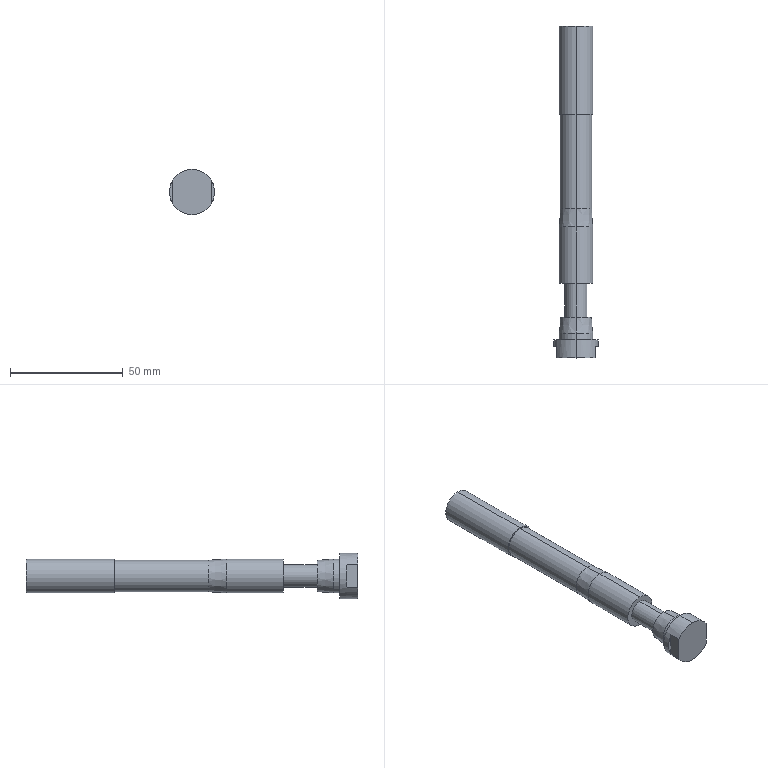Part | STEP file | 0217_203_Shaft | 1 solid | 30 faces | box 20 x 147 x 20 mm | volume 23227 mm3 | cylinder 14 | plane 10 | cone 6 | commonest cylinder face diameters 15 x6 6.8 x2 10 x2 14 x2 20 x2